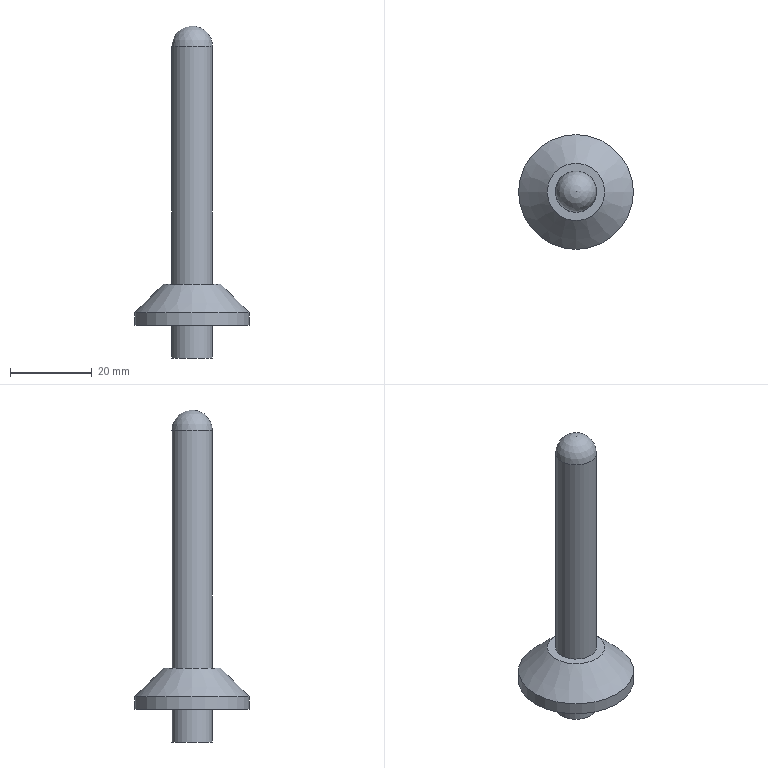Part | NX | features CYLINDER 3, BLEND 1, CHAMFER 1, DATUM_CSYS 1, UNITE 1 | 1 solid | 10 faces | box 28 x 28 x 81 mm | volume 8685 mm3 | plane 4 | cylinder 4 | cone 1 | sphere 1 | commonest cylinder face diameters 10 x2 24 x1 28 x1
STEP:
#1=CARTESIAN_POINT('',(5.,0.,18.));
#2=VERTEX_POINT('',#1);
#3=CARTESIAN_POINT('',(0.,0.,18.));
#4=DIRECTION('',(0.,0.,1.));
#5=DIRECTION('',(1.,0.,0.));
#6=AXIS2_PLACEMENT_3D('',#3,#4,#5);
#7=CIRCLE('',#6,5.);
#8=EDGE_CURVE('',#2,#2,#7,.F.);
#9=ORIENTED_EDGE('',*,*,#8,.T.);
#10=EDGE_LOOP('',(#9));
#11=FACE_BOUND('',#10,.T.);
#12=CARTESIAN_POINT('',(7.,0.,18.));
#13=VERTEX_POINT('',#12);
#14=CARTESIAN_POINT('',(0.,0.,18.));
#15=DIRECTION('',(0.,0.,1.));
#16=DIRECTION('',(1.,0.,0.));
#17=AXIS2_PLACEMENT_3D('',#14,#15,#16);
#18=CIRCLE('',#17,7.);
#19=EDGE_CURVE('',#13,#13,#18,.T.);
#20=ORIENTED_EDGE('',*,*,#19,.T.);
#21=EDGE_LOOP('',(#20));
#22=FACE_BOUND('',#21,.T.);
#23=CARTESIAN_POINT('',(0.,0.,18.));
#24=DIRECTION('',(0.,0.,1.));
#25=DIRECTION('',(1.,0.,0.));
#26=AXIS2_PLACEMENT_3D('',#23,#24,#25);
#27=PLANE('',#26);
#28=ADVANCED_FACE('',(#11,#22),#27,.T.);
#29=CARTESIAN_POINT('',(12.,0.,8.));
#30=VERTEX_POINT('',#29);
#31=CARTESIAN_POINT('',(0.,0.,8.));
#32=DIRECTION('',(0.,0.,1.));
#33=DIRECTION('',(1.,0.,0.));
#34=AXIS2_PLACEMENT_3D('',#31,#32,#33);
#35=CIRCLE('',#34,12.);
#36=EDGE_CURVE('',#30,#30,#35,.T.);
#37=ORIENTED_EDGE('',*,*,#36,.T.);
#38=EDGE_LOOP('',(#37));
#39=FACE_BOUND('',#38,.T.);
#40=CARTESIAN_POINT('',(14.,0.,8.));
#41=VERTEX_POINT('',#40);
#42=CARTESIAN_POINT('',(0.,0.,8.));
#43=DIRECTION('',(0.,0.,1.));
#44=DIRECTION('',(1.,0.,0.));
#45=AXIS2_PLACEMENT_3D('',#42,#43,#44);
#46=CIRCLE('',#45,14.);
#47=EDGE_CURVE('',#41,#41,#46,.T.);
#48=ORIENTED_EDGE('',*,*,#47,.F.);
#49=EDGE_LOOP('',(#48));
#50=FACE_BOUND('',#49,.T.);
#51=CARTESIAN_POINT('',(0.,0.,8.));
#52=DIRECTION('',(0.,0.,-1.));
#53=DIRECTION('',(-1.,0.,0.));
#54=AXIS2_PLACEMENT_3D('',#51,#52,#53);
#55=PLANE('',#54);
#56=ADVANCED_FACE('',(#39,#50),#55,.T.);
#57=CARTESIAN_POINT('',(14.,0.,11.));
#58=VERTEX_POINT('',#57);
#59=CARTESIAN_POINT('',(0.,0.,11.));
#60=DIRECTION('',(0.,0.,1.));
#61=DIRECTION('',(1.,0.,0.));
#62=AXIS2_PLACEMENT_3D('',#59,#60,#61);
#63=CIRCLE('',#62,14.);
#64=EDGE_CURVE('',#58,#58,#63,.F.);
#65=ORIENTED_EDGE('',*,*,#64,.T.);
#66=EDGE_LOOP('',(#65));
#67=FACE_BOUND('',#66,.T.);
#68=ORIENTED_EDGE('',*,*,#47,.T.);
#69=EDGE_LOOP('',(#68));
#70=FACE_BOUND('',#69,.T.);
#71=CARTESIAN_POINT('',(0.,0.,8.));
#72=DIRECTION('',(0.,0.,1.));
#73=DIRECTION('',(1.,0.,0.));
#74=AXIS2_PLACEMENT_3D('',#71,#72,#73);
#75=CYLINDRICAL_SURFACE('',#74,14.);
#76=ADVANCED_FACE('',(#67,#70),#75,.T.);
#77=ORIENTED_EDGE('',*,*,#19,.F.);
#78=EDGE_LOOP('',(#77));
#79=FACE_BOUND('',#78,.T.);
#80=ORIENTED_EDGE('',*,*,#64,.F.);
#81=EDGE_LOOP('',(#80));
#82=FACE_BOUND('',#81,.T.);
#83=CARTESIAN_POINT('',(0.,0.,11.));
#84=DIRECTION('',(0.,0.,-1.));
#85=DIRECTION('',(-1.,0.,0.));
#86=AXIS2_PLACEMENT_3D('',#83,#84,#85);
#87=CONICAL_SURFACE('',#86,14.,0.7854);
#88=ADVANCED_FACE('',(#79,#82),#87,.T.);
#89=CARTESIAN_POINT('',(5.,0.,11.));
#90=VERTEX_POINT('',#89);
#91=CARTESIAN_POINT('',(0.,0.,11.));
#92=DIRECTION('',(0.,0.,1.));
#93=DIRECTION('',(1.,0.,0.));
#94=AXIS2_PLACEMENT_3D('',#91,#92,#93);
#95=CIRCLE('',#94,5.);
#96=EDGE_CURVE('',#90,#90,#95,.T.);
#97=ORIENTED_EDGE('',*,*,#96,.T.);
#98=EDGE_LOOP('',(#97));
#99=FACE_BOUND('',#98,.T.);
#100=CARTESIAN_POINT('',(12.,0.,11.));
#101=VERTEX_POINT('',#100);
#102=CARTESIAN_POINT('',(0.,0.,11.));
#103=DIRECTION('',(0.,0.,-1.));
#104=DIRECTION('',(1.,0.,0.));
#105=AXIS2_PLACEMENT_3D('',#102,#103,#104);
#106=CIRCLE('',#105,12.);
#107=EDGE_CURVE('',#101,#101,#106,.F.);
#108=ORIENTED_EDGE('',*,*,#107,.F.);
#109=EDGE_LOOP('',(#108));
#110=FACE_BOUND('',#109,.T.);
#111=CARTESIAN_POINT('',(0.,0.,11.));
#112=DIRECTION('',(0.,0.,1.));
#113=DIRECTION('',(1.,0.,0.));
#114=AXIS2_PLACEMENT_3D('',#111,#112,#113);
#115=PLANE('',#114);
#116=ADVANCED_FACE('',(#99,#110),#115,.F.);
#117=ORIENTED_EDGE('',*,*,#107,.T.);
#118=EDGE_LOOP('',(#117));
#119=FACE_BOUND('',#118,.T.);
#120=ORIENTED_EDGE('',*,*,#36,.F.);
#121=EDGE_LOOP('',(#120));
#122=FACE_BOUND('',#121,.T.);
#123=CARTESIAN_POINT('',(0.,0.,8.));
#124=DIRECTION('',(0.,0.,1.));
#125=DIRECTION('',(1.,0.,0.));
#126=AXIS2_PLACEMENT_3D('',#123,#124,#125);
#127=CYLINDRICAL_SURFACE('',#126,12.);
#128=ADVANCED_FACE('',(#119,#122),#127,.F.);
#129=CARTESIAN_POINT('',(5.,0.,0.));
#130=VERTEX_POINT('',#129);
#131=CARTESIAN_POINT('',(0.,0.,0.));
#132=DIRECTION('',(0.,0.,1.));
#133=DIRECTION('',(1.,0.,0.));
#134=AXIS2_PLACEMENT_3D('',#131,#132,#133);
#135=CIRCLE('',#134,5.);
#136=EDGE_CURVE('',#130,#130,#135,.T.);
#137=ORIENTED_EDGE('',*,*,#136,.F.);
#138=EDGE_LOOP('',(#137));
#139=FACE_BOUND('',#138,.T.);
#140=CARTESIAN_POINT('',(0.,0.,0.));
#141=DIRECTION('',(0.,0.,-1.));
#142=DIRECTION('',(-1.,0.,0.));
#143=AXIS2_PLACEMENT_3D('',#140,#141,#142);
#144=PLANE('',#143);
#145=ADVANCED_FACE('',(#139),#144,.T.);
#146=ORIENTED_EDGE('',*,*,#136,.T.);
#147=EDGE_LOOP('',(#146));
#148=FACE_BOUND('',#147,.T.);
#149=ORIENTED_EDGE('',*,*,#96,.F.);
#150=EDGE_LOOP('',(#149));
#151=FACE_BOUND('',#150,.T.);
#152=CARTESIAN_POINT('',(0.,0.,0.));
#153=DIRECTION('',(0.,0.,1.));
#154=DIRECTION('',(1.,0.,0.));
#155=AXIS2_PLACEMENT_3D('',#152,#153,#154);
#156=CYLINDRICAL_SURFACE('',#155,5.);
#157=ADVANCED_FACE('',(#148,#151),#156,.T.);
#158=ORIENTED_EDGE('',*,*,#8,.F.);
#159=EDGE_LOOP('',(#158));
#160=FACE_BOUND('',#159,.T.);
#161=CARTESIAN_POINT('',(5.,0.,76.));
#162=VERTEX_POINT('',#161);
#163=CARTESIAN_POINT('',(0.,0.,76.));
#164=DIRECTION('',(0.,0.,1.));
#165=DIRECTION('',(1.,0.,0.));
#166=AXIS2_PLACEMENT_3D('',#163,#164,#165);
#167=CIRCLE('',#166,5.);
#168=EDGE_CURVE('',#162,#162,#167,.F.);
#169=ORIENTED_EDGE('',*,*,#168,.T.);
#170=EDGE_LOOP('',(#169));
#171=FACE_BOUND('',#170,.T.);
#172=CARTESIAN_POINT('',(0.,0.,0.));
#173=DIRECTION('',(0.,0.,1.));
#174=DIRECTION('',(1.,0.,0.));
#175=AXIS2_PLACEMENT_3D('',#172,#173,#174);
#176=CYLINDRICAL_SURFACE('',#175,5.);
#177=ADVANCED_FACE('',(#160,#171),#176,.T.);
#178=ORIENTED_EDGE('',*,*,#168,.F.);
#179=EDGE_LOOP('',(#178));
#180=FACE_BOUND('',#179,.T.);
#181=CARTESIAN_POINT('',(0.,0.,76.));
#182=DIRECTION('',(0.,0.,1.));
#183=DIRECTION('',(1.,0.,0.));
#184=AXIS2_PLACEMENT_3D('',#181,#182,#183);
#185=SPHERICAL_SURFACE('',#184,5.);
#186=ADVANCED_FACE('',(#180),#185,.T.);
#187=CLOSED_SHELL('',(#28,#56,#76,#88,#116,#128,#145,#157,#177,#186));
#188=MANIFOLD_SOLID_BREP('',#187);
#189=(LENGTH_UNIT()NAMED_UNIT(*)SI_UNIT(.MILLI.,.METRE.));
#190=UNCERTAINTY_MEASURE_WITH_UNIT(LENGTH_MEASURE(0.00001),#189,'','');
#191=(NAMED_UNIT(*)PLANE_ANGLE_UNIT()SI_UNIT($,.RADIAN.));
#192=(NAMED_UNIT(*)SI_UNIT($,.STERADIAN.)SOLID_ANGLE_UNIT());
#193=(GEOMETRIC_REPRESENTATION_CONTEXT(3)GLOBAL_UNCERTAINTY_ASSIGNED_CONTEXT((#190))GLOBAL_UNIT_ASSIGNED_CONTEXT((#189,#191,#192))REPRESENTATION_CONTEXT('',''));
#194=ADVANCED_BREP_SHAPE_REPRESENTATION('',(#188),#193);